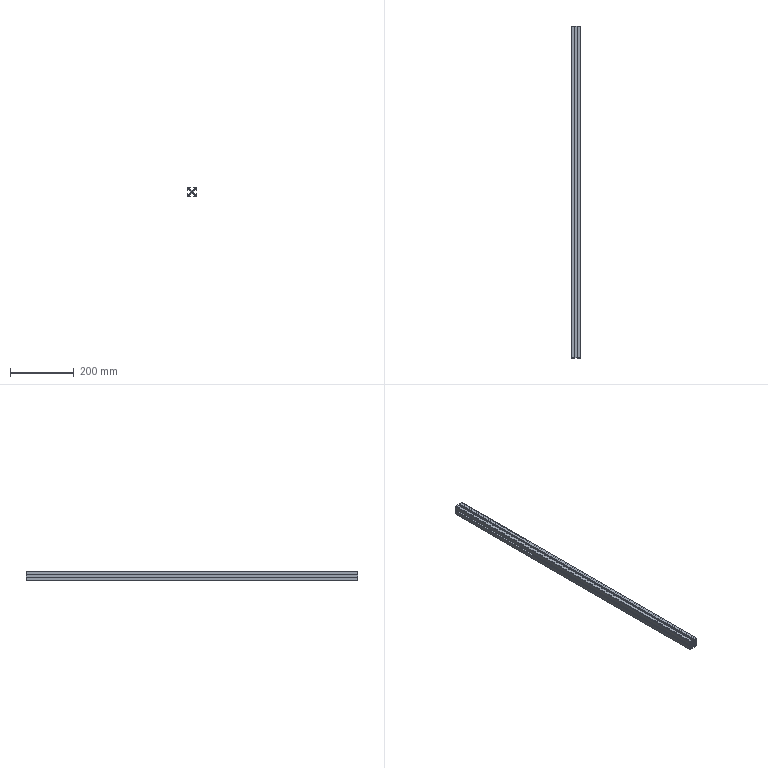Part | STEP file | 08-04 Guard bracket 4 | 1 solid | 68 faces | box 30 x 1040 x 30 mm | volume 439641 mm3 | plane 54 | cylinder 14 | commonest cylinder face diameters 6 x10 2 x4